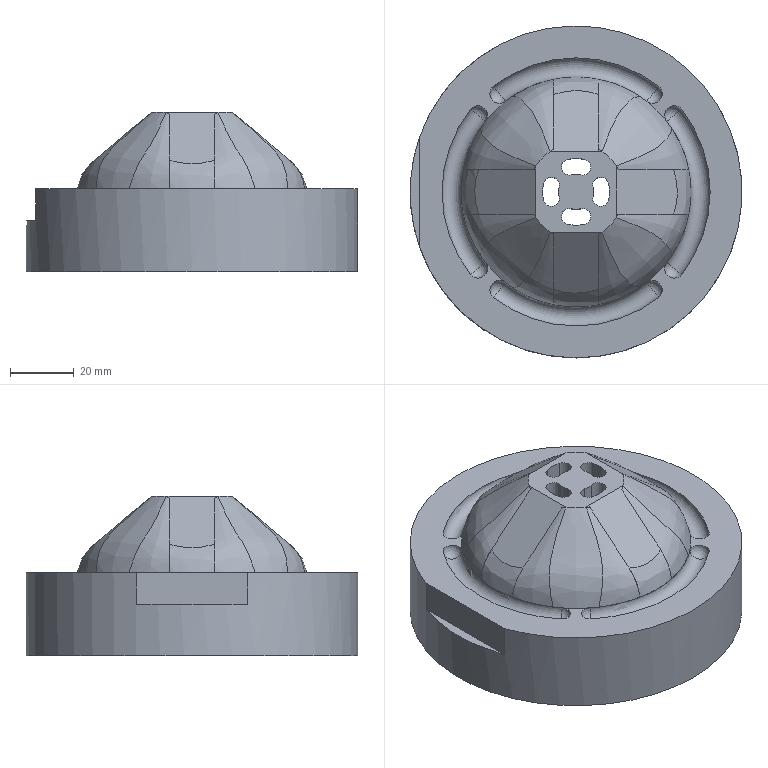NC program | NX | posted with a generic post | part box 104 x 104 x 49.86 mm
Lines 1 to 886 of 41131:
N10 G17 G21 G94 G90
(CAVITY_MILL , TOOL : D20R0.8)
N12 T00 M6
N14 G54
N16 G17 G0 G90 X-25.307 Y60.87 S2992 M3
N18 G43 Z20. H0
N20 Z-0.394
N22 G94 G1 Z-0.594 F1250.
N24 X-20.333 Y48.906
N26 G2 X26.248 Y46.008 R52.973 F2500.
N28 X51.613 Y-11.894 R52.996
N30 G1 X50.48 Y-16.058
N32 G2 X-38.754 Y-36.105 R52.977
N34 X-43.498 Y-30.233 R58.963
N36 X-20.333 Y48.906 R52.973
N38 G1 X-15.741 Y37.863
N40 G2 X20.32 Y35.62 R41.013
N42 X40.006 Y-8.998 R41.036
N44 G1 X39.011 Y-12.657
N46 G2 X-29.978 Y-27.979 R41.017
N48 X-33.704 Y-23.369 R47.003
N50 X-15.741 Y37.863 R41.013
N52 G1 X-11.15 Y26.819
N54 G2 X14.392 Y25.233 R29.053
N56 X28.389 Y-6.14 R29.076
N58 G1 X27.553 Y-9.214
N60 G2 X-21.203 Y-19.853 R29.057
N62 X-23.909 Y-16.505 R35.043
N64 X-11.15 Y26.819 R29.053
N66 G1 X-10.379 Y22.906
N68 G2 X-8.681 Y23.071 R8.786
N70 G1 X8.658
N72 G2 X13.35 Y21.729 R8.871
N74 X21.749 Y13.316 R26.19
N76 X23.071 Y8.681 R8.788
N78 G1 Y-8.663
N80 G2 X21.734 Y-13.342 R8.857
N82 X13.308 Y-21.754 R26.163
N84 X8.685 Y-23.071 R8.772
N86 G1 X-8.658
N88 G2 X-13.35 Y-21.729 R8.871
N90 X-21.749 Y-13.316 R26.19
N92 X-23.071 Y-8.681 R8.788
N94 G1 Y8.686
N96 G2 X-21.754 Y13.309 R8.769
N98 X-13.315 Y21.75 R26.175
N100 X-10.379 Y22.906 R8.786
N102 G3 X-4.863 Y31.126 R7.
N104 G1 X-11.113 Y71.102
N106 Z-0.394
N108 G0 Z0.3
N110 G1 X-25.307 Y60.87 F5000.
N112 G0 Z-0.988
N114 G1 Z-1.188 F1250.
N116 X-20.353 Y48.929
N118 G2 X9.52 Y52.133 R53.179 F2500.
N120 X29.214 Y44.212 R53.094
N122 X40.074 Y34.681 R53.73
N124 X52.332 Y-8.325 R53.011
N126 G1 X51.585 Y-12.117
N128 X50.507 Y-16.064
N130 G2 X-52.784 Y4.709 R52.998
N132 X-39.002 Y35.87 R52.95
N134 X-34.07 Y40.592 R54.178
N136 X-25.024 Y46.719 R56.698
N138 X-20.353 Y48.929 R53.179
N140 G1 X-15.77 Y37.882
N142 G2 X7.375 Y40.367 R41.219
N144 X22.614 Y34.238 R41.134
N146 X31.038 Y26.846 R41.77
N148 X40.553 Y-6.242 R41.051
N150 G1 X39.934 Y-9.381
N152 X39.039 Y-12.659
N154 G2 X-40.871 Y3.647 R41.038
N156 X-30.202 Y27.77 R40.99
N158 X-26.399 Y31.416 R42.218
N160 X-19.347 Y36.193 R44.738
N162 X-15.77 Y37.882 R41.219
N164 G1 X-11.188 Y26.835
N166 G2 X5.23 Y28.601 R29.259
N168 X16.014 Y24.264 R29.174
N170 X22.002 Y19.011 R29.81
N172 X28.766 Y-4.196 R29.091
N174 G1 X28.283 Y-6.645
N176 X27.582 Y-9.212
N178 G2 X-28.959 Y2.586 R29.078
N180 X-21.402 Y19.67 R29.03
N182 X-18.728 Y22.24 R30.258
N184 X-13.67 Y25.666 R32.778
N186 X-11.188 Y26.835 R29.259
N188 G1 X-10.509 Y23.631
N190 G2 X-6.468 Y23.779 R11.801
N192 G1 X6.453
N194 G2 X13.099 Y22.76 R11.911
N196 X22.76 Y13.099 R26.82
N198 X23.779 Y6.468 R11.801
N200 G1 Y-6.453
N202 G2 X22.76 Y-13.099 R11.911
N204 X13.099 Y-22.76 R26.82
N206 X6.468 Y-23.779 R11.801
N208 G1 X-6.453
N210 G2 X-13.099 Y-22.76 R11.911
N212 X-22.76 Y-13.099 R26.82
N214 X-23.779 Y-6.468 R11.801
N216 G1 Y6.453
N218 G2 X-22.76 Y13.099 R11.911
N220 X-13.099 Y22.76 R26.82
N222 X-10.509 Y23.631 R11.801
N224 G3 X-5.111 Y31.93 R7.
N226 G1 X-11.371 Y71.083
N228 Z-0.988
N230 G0 Z-0.294
N232 G1 X-25.307 Y60.87 F5000.
N234 G0 Z-1.582
N236 G1 Z-1.782 F1250.
N238 X-20.353 Y48.929
N240 G2 X9.52 Y52.133 R53.179 F2500.
N242 X29.214 Y44.212 R53.094
N244 X40.074 Y34.681 R53.73
N246 X52.332 Y-8.325 R53.011
N248 G1 X51.585 Y-12.117
N250 X50.507 Y-16.064
N252 G2 X-52.784 Y4.709 R52.998
N254 X-39.002 Y35.87 R52.95
N256 X-34.07 Y40.592 R54.178
N258 X-25.024 Y46.719 R56.698
N260 X-20.353 Y48.929 R53.179
N262 G1 X-15.77 Y37.882
N264 G2 X7.375 Y40.367 R41.219
N266 X22.614 Y34.238 R41.134
N268 X31.038 Y26.846 R41.77
N270 X40.553 Y-6.242 R41.051
N272 G1 X39.934 Y-9.381
N274 X39.039 Y-12.659
N276 G2 X37.457 Y-16.768 R41.038
N278 G1 X26.542 Y-11.88
N280 G3 X26.879 Y-6.148 R14.969
N282 G1 Y6.149
N284 G3 X26.553 Y11.841 R14.936
N286 G2 X28.766 Y-4.196 R29.091
N288 G1 X28.283 Y-6.645
N290 X27.582 Y-9.212
N292 G2 X26.542 Y-11.88 R29.077
N294 G1 X37.457 Y-16.768
N296 G2 X-16.701 Y-37.478 R41.038
N298 G1 X-11.833 Y-26.554
N300 G3 X-6.148 Y-26.879 R14.969
N302 G1 X6.149
N304 G3 X11.847 Y-26.551 R14.936
N306 G1 X21.681 Y-21.708
N308 X11.847 Y-26.551
N310 G2 X-11.833 Y-26.554 R29.078
N312 G1 X-21.693 Y-21.688
N314 X-11.833 Y-26.554
N316 X-16.701 Y-37.478
N318 G2 X-40.871 Y3.647 R41.038
N320 X-37.471 Y16.722 R40.99
N322 G1 X-26.55 Y11.846
N324 G3 X-26.879 Y6.148 R14.969
N326 G1 Y-6.149
N328 G3 X-26.555 Y-11.831 R14.936
N330 G2 X-28.959 Y2.586 R29.078
N332 X-26.55 Y11.846 R29.03
N334 G1 X-21.69 Y21.692
N336 X-26.55 Y11.846
N338 X-37.471 Y16.722
N340 G2 X-30.202 Y27.77 R40.99
N342 X-26.399 Y31.416 R42.218
N344 X-19.347 Y36.193 R44.738
N346 X-15.77 Y37.882 R41.219
N348 G1 X-11.188 Y26.835
N350 G2 X5.23 Y28.601 R29.259
N352 X11.825 Y26.558 R29.174
N354 G1 X21.687 Y21.695
N356 X11.825 Y26.558
N358 G3 X6.146 Y26.879 R14.907
N360 G1 X-6.149
N362 G3 X-11.848 Y26.551 R14.936
N364 G1 X-11.257 Y24.233
N366 G2 X-6.317 Y24.487 R12.544
N368 G1 X6.316
N370 G2 X13.099 Y23.608 R12.515
N372 X19.538 Y18.556 R25.887
N374 X23.608 Y13.099 R25.007
N376 X24.487 Y6.317 R12.544
N378 G1 Y-6.316
N380 G2 X23.608 Y-13.099 R12.577
N382 X18.556 Y-19.538 R25.887
N384 X13.099 Y-23.608 R25.007
N386 X6.317 Y-24.487 R12.544
N388 G1 X-6.316
N390 G2 X-13.099 Y-23.608 R12.577
N392 X-19.538 Y-18.556 R25.887
N394 X-23.608 Y-13.099 R25.007
N396 X-24.487 Y-6.317 R12.544
N398 G1 Y6.316
N400 G2 X-23.608 Y13.099 R12.577
N402 X-18.556 Y19.538 R25.887
N404 X-13.099 Y23.608 R25.007
N406 X-11.257 Y24.233 R12.544
N408 G1 X-11.848 Y26.551
N410 G2 X-11.188 Y26.835 R29.259
N412 G3 X-7.404 Y35.983 R7.
N414 G1 X-14.495 Y70.513
N416 Z-1.582
N418 G0 Z-0.888
N420 G1 X-25.307 Y60.87 F5000.
N422 G0 Z-2.176
N424 G1 Z-2.376 F1250.
N426 X-20.353 Y48.929
N428 G2 X9.52 Y52.133 R53.179 F2500.
N430 X29.214 Y44.212 R53.094
N432 X40.074 Y34.681 R53.73
N434 X52.332 Y-8.325 R53.011
N436 G1 X51.585 Y-12.117
N438 X50.507 Y-16.064
N440 G2 X-52.784 Y4.709 R52.998
N442 X-39.002 Y35.87 R52.95
N444 X-34.07 Y40.592 R54.178
N446 X-25.024 Y46.719 R56.698
N448 X-20.353 Y48.929 R53.179
N450 G1 X-15.77 Y37.882
N452 G2 X7.375 Y40.367 R41.219
N454 X12.246 Y39.163 R41.134
N456 G1 X8.672 Y27.749
N458 G3 X6.039 Y27.587 R14.932
N460 G1 X-6.07
N462 G3 X-8.791 Y27.708 R18.71
N464 G2 X5.23 Y28.601 R29.259
N466 X8.672 Y27.749 R29.174
N468 G1 X21.735 Y21.834
N470 X8.672 Y27.749
N472 X12.246 Y39.163
N474 G2 X22.614 Y34.238 R41.134
N476 X31.038 Y26.846 R41.77
N478 X40.553 Y-6.242 R41.051
N480 G1 X39.934 Y-9.381
N482 X39.288 Y-11.745
N484 X27.751 Y-8.594
N486 G3 X27.587 Y-6.039 R14.932
N488 G1 Y6.07
N490 G3 X27.708 Y8.801 R18.71
N492 G2 X28.766 Y-4.196 R29.091
N494 G1 X28.283 Y-6.645
N496 X27.751 Y-8.594
N498 X39.288 Y-11.745
N500 X39.039 Y-12.659
N502 G2 X-12.233 Y-39.165 R41.038
N504 G1 X-8.667 Y-27.749
N506 G3 X-6.039 Y-27.587 R14.932
N508 G1 X6.07
N510 G3 X8.806 Y-27.708 R18.71
N512 G1 X21.871 Y-21.699
N514 X8.806 Y-27.708
N516 G2 X-8.667 Y-27.749 R29.078
N518 G1 X-21.729 Y-21.84
N520 X-8.667 Y-27.749
N522 X-12.233 Y-39.165
N524 G2 X-40.871 Y3.647 R41.038
N526 X-39.163 Y12.248 R40.99
N528 G1 X-27.749 Y8.677
N530 G3 X-27.587 Y6.039 R14.932
N532 G1 Y-6.07
N534 G3 X-27.708 Y-8.8 R18.71
N536 G1 X-25.317 Y-8.731
N538 G2 X-25.195 Y-6.216 R16.318
N540 G1 Y6.226
N542 G2 X-24.014 Y13.927 R12.54
N544 X-14.394 Y23.741 R31.514
N546 X-10.725 Y25.137 R9.325
N548 X-6.216 Y25.195 R16.318
N550 G1 X6.226
N552 G2 X13.927 Y24.014 R12.54
N554 X23.741 Y14.394 R31.514
N556 X25.137 Y10.725 R9.325
N558 X25.195 Y6.216 R16.318
N560 G1 Y-6.226
N562 G2 X24.014 Y-13.927 R12.54
N564 X14.394 Y-23.741 R31.514
N566 X10.725 Y-25.137 R9.325
N568 X6.216 Y-25.195 R16.318
N570 G1 X-6.226
N572 G2 X-13.927 Y-24.014 R12.54
N574 X-23.741 Y-14.394 R31.514
N576 X-25.137 Y-10.725 R9.325
N578 X-25.317 Y-8.731 R16.318
N580 G1 X-27.708 Y-8.8
N582 G2 X-28.959 Y2.586 R29.078
N584 X-27.749 Y8.677 R29.03
N586 G1 X-21.836 Y21.731
N588 X-27.749 Y8.677
N590 X-39.163 Y12.248
N592 G2 X-30.202 Y27.77 R40.99
N594 X-26.399 Y31.416 R42.218
N596 X-19.347 Y36.193 R44.738
N598 X-15.77 Y37.882 R41.219
N600 G3 X-11.987 Y47.03 R7.
N602 G1 X-21.038 Y68.847
N604 Z-2.176
N606 G0 Z-1.482
N608 G1 X-25.307 Y60.87 F5000.
N610 G0 Z-2.77
N612 G1 Z-2.97 F1250.
N614 X-20.353 Y48.929
N616 G2 X9.52 Y52.133 R53.179 F2500.
N618 X29.214 Y44.212 R53.094
N620 X40.074 Y34.681 R53.73
N622 X52.332 Y-8.325 R53.011
N624 G1 X51.585 Y-12.117
N626 X50.507 Y-16.064
N628 G2 X-52.784 Y4.709 R52.998
N630 X-39.002 Y35.87 R52.95
N632 X-34.07 Y40.592 R54.178
N634 X-25.024 Y46.719 R56.698
N636 X-20.353 Y48.929 R53.179
N638 G1 X-15.77 Y37.882
N640 G2 X7.375 Y40.367 R41.219
N642 X9.127 Y40.006 R41.134
N644 G1 X6.46 Y28.348
N646 G3 X6.034 Y28.295 R16.746
N648 G1 X-6.028
N650 G3 X-6.452 Y28.342 R18.538
N652 G2 X5.23 Y28.601 R29.259
N654 X6.46 Y28.348 R29.174
N656 G1 X21.906 Y21.889
N658 X6.46 Y28.348
N660 X9.127 Y40.006
N662 G2 X22.614 Y34.238 R41.134
N664 X31.038 Y26.846 R41.77
N666 X40.553 Y-6.242 R41.051
N668 G1 X40.072 Y-8.683
N670 X28.337 Y-6.37
N672 G3 X28.295 Y-6.034 R16.746
N674 G1 Y6.028
N676 G3 X28.344 Y6.465 R18.538
N678 G2 X28.766 Y-4.196 R29.091
N680 G1 X28.337 Y-6.37
N682 X40.072 Y-8.683
N684 X39.934 Y-9.381
N686 X39.039 Y-12.659
N688 G2 X-9.106 Y-40.008 R41.038
N690 G1 X-6.451 Y-28.347
N692 G3 X-6.034 Y-28.295 R16.746
N694 G1 X6.028
N696 G3 X6.47 Y-28.344 R18.538
N698 G1 X21.931 Y-21.863
N700 X6.47 Y-28.344
N702 G2 X-6.451 Y-28.347 R29.077
N704 G1 X-21.895 Y-21.899
N706 X-6.451 Y-28.347
N708 X-9.106 Y-40.008
N710 G2 X-40.871 Y3.647 R41.038
N712 X-40.009 Y9.117 R40.99
N714 G1 X-28.348 Y6.46
N716 G3 X-28.295 Y6.034 R16.746
N718 G1 Y-6.028
N720 G3 X-28.344 Y-6.467 R18.538
N722 G1 X-25.964 Y-6.704
N724 G2 X-25.903 Y-6.181 R16.146
N726 G1 Y6.203
N728 G2 X-25.234 Y13.099 R14.354
N730 X-24.247 Y14.969 R7.318
N732 G1 X-23.532 Y15.949
N734 G2 X-15.106 Y24.14 R34.922
N736 X-10.846 Y25.842 R10.411
N738 X-6.181 Y25.903 R16.146
N740 G1 X6.203
N742 G2 X13.099 Y25.234 R14.354
N744 X14.969 Y24.247 R7.318
N746 G1 X15.949 Y23.532
N748 G2 X24.14 Y15.106 R34.922
N750 X25.842 Y10.846 R10.411
N752 X25.903 Y6.181 R16.146
N754 G1 Y-6.203
N756 G2 X25.234 Y-13.099 R14.354
N758 X24.247 Y-14.969 R7.318
N760 G1 X23.532 Y-15.949
N762 G2 X15.106 Y-24.14 R34.922
N764 X10.846 Y-25.842 R10.411
N766 X6.181 Y-25.903 R16.146
N768 G1 X-6.203
N770 G2 X-13.099 Y-25.234 R14.354
N772 X-14.969 Y-24.247 R7.318
N774 G1 X-15.949 Y-23.532
N776 G2 X-24.14 Y-15.106 R34.922
N778 X-25.842 Y-10.846 R10.411
N780 X-25.964 Y-6.704 R16.146
N782 G1 X-28.344 Y-6.467
N784 G2 X-28.959 Y2.586 R29.078
N786 X-28.348 Y6.46 R29.03
N788 G1 X-21.901 Y21.891
N790 X-28.348 Y6.46
N792 X-40.009 Y9.117
N794 G2 X-30.202 Y27.77 R40.99
N796 X-26.399 Y31.416 R42.218
N798 X-19.347 Y36.193 R44.738
N800 X-15.77 Y37.882 R41.219
N802 G3 X-11.987 Y47.03 R7.
N804 G1 X-21.038 Y68.847
N806 Z-2.77
N808 G0 Z-2.076
N810 G1 X-25.307 Y60.87 F5000.
N812 G0 Z-3.364
N814 G1 Z-3.564 F1250.
N816 X-20.353 Y48.929
N818 G2 X9.52 Y52.133 R53.179 F2500.
N820 X29.214 Y44.212 R53.094
N822 X40.074 Y34.681 R53.73
N824 X52.332 Y-8.325 R53.011
N826 G1 X51.585 Y-12.117
N828 X50.507 Y-16.064
N830 G2 X-52.784 Y4.709 R52.998
N832 X-39.002 Y35.87 R52.95
N834 X-34.07 Y40.592 R54.178
N836 X-25.024 Y46.719 R56.698
N838 X-20.353 Y48.929 R53.179
N840 G1 X-15.77 Y37.882
N842 G2 X2.776 Y40.936 R41.219
N844 G1 X1.978 Y29.003
N846 X-1.929
N848 G2 X1.978 Y29.003 R29.259
N850 G1 X11.177 Y28.938
N852 G2 X15.18 Y27.705 R16.41
N854 X15.436 Y27.569 R2.392
N856 X27.569 Y15.436 R36.475
N858 X27.706 Y15.178 R2.392
N860 X28.934 Y11.188 R16.475
N862 X29.815 Y11.152 R9.2
N864 G3 X24.087 Y20.819 R31.851
N866 X17.537 Y26.566 R32.57
N868 X11.141 Y29.818 R31.934
N870 G2 X11.177 Y28.938 R9.2
N872 G1 X1.978 Y29.003
N874 X2.776 Y40.936
N876 G2 X7.375 Y40.367 R41.219
N878 X22.614 Y34.238 R41.134
N880 X31.038 Y26.846 R41.77
N882 X40.935 Y-2.799 R41.051
N884 G1 X29.003 Y-1.983
N886 Y1.988
N888 G2 X29.003 Y-1.983 R29.091
N890 G1 X28.937 Y-11.182
N892 G2 X27.705 Y-15.18 R16.41
N894 X27.569 Y-15.436 R2.392
N896 X15.436 Y-27.569 R36.475
N898 X15.178 Y-27.706 R2.392
N900 X11.213 Y-28.93 R16.475
N902 X11.178 Y-29.807 R9.2
N904 G3 X29.825 Y-11.146 R31.838
N906 G2 X28.937 Y-11.182 R9.2
N908 G1 X29.003 Y-1.983
N910 X40.935 Y-2.799
N912 G2 X40.553 Y-6.242 R41.051
N914 G1 X39.934 Y-9.381
N916 X39.039 Y-12.659
N918 G2 X-2.831 Y-40.934 R41.038
N920 G1 X-2.005 Y-29.003
N922 X2.013
N924 G2 X-2.005 Y-29.003 R29.077
N926 G1 X-2.831 Y-40.934
N928 G2 X-40.934 Y2.864 R41.038
N930 G1 X-29.003 Y2.031
N932 Y-2.02
N934 X-29.802 Y-11.185
N936 G3 X-11.17 Y-29.807 R31.838
N938 G2 X-11.205 Y-28.933 R9.2
N940 X-15.18 Y-27.705 R16.41
N942 X-15.436 Y-27.569 R2.392
N944 X-27.569 Y-15.436 R36.475
N946 X-27.706 Y-15.178 R2.392
N948 X-28.929 Y-11.22 R16.475
N950 X-29.802 Y-11.185 R9.2
N952 G1 X-29.003 Y-2.02
N954 X-26.611
N956 Y6.186
N958 G2 X-25.527 Y14.19 R14.018
N960 X-14.19 Y25.528 R34.083
N962 X-6.169 Y26.611 R14.083
N964 G1 X6.186
N966 G2 X14.19 Y25.527 R14.018
N968 X25.528 Y14.19 R34.083
N970 X26.611 Y6.169 R14.083
N972 G1 Y-6.186
N974 G2 X25.527 Y-14.19 R14.018
N976 X14.19 Y-25.528 R34.083
N978 X6.169 Y-26.611 R14.083
N980 G1 X-6.186
N982 G2 X-14.19 Y-25.527 R14.018
N984 X-25.528 Y-14.19 R34.083
N986 X-26.611 Y-6.169 R14.083
N988 G1 Y-2.02
N990 X-29.003
N992 G2 X-29.003 Y2.031 R29.077
N994 G1 X-28.929 Y11.23
N996 G2 X-27.705 Y15.18 R16.41
N998 X-27.569 Y15.436 R2.392
N1000 X-15.436 Y27.569 R36.475
N1002 X-15.178 Y27.706 R2.392
N1004 X-11.129 Y28.945 R16.475
N1006 X-11.091 Y29.837 R9.2
N1008 G3 X-14.98 Y28.095 R32.019
N1010 X-20.498 Y24.358 R35.538
N1012 X-23.433 Y21.539 R33.018
N1014 X-29.8 Y11.196 R31.79
N1016 G2 X-28.929 Y11.23 R9.2
N1018 G1 X-29.003 Y2.031
N1020 X-40.934 Y2.864
N1022 G2 X-40.871 Y3.647 R41.038
N1024 X-30.202 Y27.77 R40.99
N1026 X-26.399 Y31.416 R42.218
N1028 X-19.347 Y36.193 R44.738
N1030 X-15.77 Y37.882 R41.219
N1032 G3 X-11.987 Y47.03 R7.
N1034 G1 X-21.038 Y68.847
N1036 Z-3.364
N1038 G0 Z-2.67
N1040 G1 X-25.307 Y60.87 F5000.
N1042 G0 Z-3.958
N1044 G1 Z-4.158 F1250.
N1046 X-20.353 Y48.929
N1048 G2 X9.52 Y52.133 R53.179 F2500.
N1050 X29.214 Y44.212 R53.094
N1052 X40.074 Y34.681 R53.73
N1054 X52.332 Y-8.325 R53.011
N1056 G1 X51.585 Y-12.117
N1058 X50.507 Y-16.064
N1060 G2 X-52.784 Y4.709 R52.998
N1062 X-39.002 Y35.87 R52.95
N1064 X-34.07 Y40.592 R54.178
N1066 X-25.024 Y46.719 R56.698
N1068 X-20.353 Y48.929 R53.179
N1070 G1 X-15.77 Y37.882
N1072 G2 X7.375 Y40.367 R41.219
N1074 X22.614 Y34.238 R41.134
N1076 X31.038 Y26.846 R41.77
N1078 X40.553 Y-6.242 R41.051
N1080 G1 X39.934 Y-9.381
N1082 X39.039 Y-12.659
N1084 G2 X37.429 Y-16.831 R41.038
N1086 G1 X29.221 Y-13.138
N1088 G3 X29.711 Y-5.993 R16.886
N1090 G1 Y5.994
N1092 G3 X29.233 Y13.099 R16.887
N1094 G2 X31.684 Y-4.698 R32.051
N1096 G1 X31.167 Y-7.322
N1098 X30.416 Y-10.07
N1100 G2 X29.221 Y-13.138 R32.037
N1102 G1 X37.429 Y-16.831
N1104 G2 X-16.759 Y-37.452 R41.038
N1106 G1 X-13.083 Y-29.237
N1108 G3 X-5.993 Y-29.711 R16.886
N1110 G1 X5.994
N1112 G3 X13.105 Y-29.231 R16.887
N1114 G2 X-13.083 Y-29.237 R32.038
N1116 G1 X-16.759 Y-37.452
N1118 G2 X-40.871 Y3.647 R41.038
N1120 X-37.445 Y16.781 R40.99
N1122 G1 X-29.233 Y13.098
N1124 G3 X-29.711 Y5.993 R16.886
N1126 G1 Y-5.994
N1128 G3 X-29.237 Y-13.086 R16.887
N1130 G2 X-31.907 Y2.849 R32.037
N1132 X-29.233 Y13.098 R31.99
N1134 G1 X-37.445 Y16.781
N1136 G2 X-30.202 Y27.77 R40.99
N1138 X-26.399 Y31.416 R42.218
N1140 X-19.347 Y36.193 R44.738
N1142 X-15.77 Y37.882 R41.219
N1144 G1 X-12.322 Y29.569
N1146 G2 X5.76 Y31.513 R32.219
N1148 X13.086 Y29.236 R32.134
N1150 G3 X5.993 Y29.711 R16.886
N1152 G1 X-5.994
N1154 G3 X-13.108 Y29.23 R16.887
N1156 G1 X-12.446 Y26.932
N1158 G2 X-6.175 Y27.319 R14.495
N1160 G1 X6.174
N1162 G2 X14.437 Y26.197 R14.494
N1164 X21.264 Y20.739 R32.312
N1166 X26.197 Y14.437 R31.95
N1168 X27.319 Y6.175 R14.495
N1170 G1 Y-6.174
N1172 G2 X26.197 Y-14.437 R14.494
N1174 X20.739 Y-21.264 R32.312
N1176 X14.437 Y-26.197 R31.95
N1178 X6.175 Y-27.319 R14.495
N1180 G1 X-6.174
N1182 G2 X-14.437 Y-26.197 R14.494
N1184 X-21.264 Y-20.739 R32.312
N1186 X-26.197 Y-14.437 R31.95
N1188 X-27.319 Y-6.175 R14.495
N1190 G1 Y6.174
N1192 G2 X-26.197 Y14.437 R14.494
N1194 X-20.739 Y21.264 R32.312
N1196 X-14.437 Y26.197 R31.95
N1198 X-12.446 Y26.932 R14.495
N1200 G1 X-13.108 Y29.23
N1202 G2 X-12.322 Y29.569 R32.219
N1204 G3 X-8.538 Y38.717 R7.
N1206 G1 X-15.489 Y70.301
N1208 Z-3.958
N1210 G0 Z-3.264
N1212 G1 X-25.307 Y60.87 F5000.
N1214 G0 Z-4.552
N1216 G1 Z-4.752 F1250.
N1218 X-20.353 Y48.929
N1220 G2 X9.52 Y52.133 R53.179 F2500.
N1222 X29.214 Y44.212 R53.094
N1224 X40.074 Y34.681 R53.73
N1226 X52.332 Y-8.325 R53.011
N1228 G1 X51.585 Y-12.117
N1230 X50.507 Y-16.064
N1232 G2 X-52.784 Y4.709 R52.998
N1234 X-39.002 Y35.87 R52.95
N1236 X-34.07 Y40.592 R54.178
N1238 X-25.024 Y46.719 R56.698
N1240 X-20.353 Y48.929 R53.179
N1242 G1 X-15.77 Y37.882
N1244 G2 X7.375 Y40.367 R41.219
N1246 X12.345 Y39.132 R41.134
N1248 G1 X9.634 Y30.55
N1250 G3 X5.993 Y30.419 R18.009
N1252 G1 X-6.024
N1254 G3 X-9.635 Y30.546 R19.375
N1256 G2 X5.76 Y31.513 R32.219
N1258 X9.634 Y30.55 R32.134
N1260 G1 X12.345 Y39.132
N1262 G2 X22.614 Y34.238 R41.134
N1264 X31.038 Y26.846 R41.77
N1266 X40.553 Y-6.242 R41.051
N1268 G1 X39.934 Y-9.381
N1270 X39.236 Y-11.937
N1272 X30.554 Y-9.566
N1274 G3 X30.419 Y-5.993 R18.009
N1276 G1 Y6.024
N1278 G3 X30.545 Y9.646 R19.375
N1280 G2 X31.684 Y-4.698 R32.051
N1282 G1 X31.167 Y-7.322
N1284 X30.554 Y-9.566
N1286 X39.236 Y-11.937
N1288 X39.039 Y-12.659
N1290 G2 X-12.334 Y-39.134 R41.038
N1292 G1 X-9.628 Y-30.55
N1294 G3 X-5.993 Y-30.419 R18.009
N1296 G1 X6.024
N1298 G3 X9.652 Y-30.545 R19.375
N1300 G2 X-9.628 Y-30.55 R32.037
N1302 G1 X-12.334 Y-39.134
N1304 G2 X-40.871 Y3.647 R41.038
N1306 X-39.132 Y12.349 R40.99
N1308 G1 X-30.549 Y9.64
N1310 G3 X-30.419 Y5.993 R18.009
N1312 G1 Y-6.024
N1314 G3 X-30.546 Y-9.644 R19.375
N1316 G1 X-28.158 Y-9.505
N1318 G2 X-28.027 Y-6.184 R16.983
N1320 G1 Y6.164
N1322 G2 X-27.106 Y14.19 R15.617
N1324 X-25.592 Y16.684 R14.657
N1326 G1 X-25.004 Y17.465
N1328 G2 X-16.054 Y26.019 R39.967
N1330 X-11.234 Y27.967 R11.749
N1332 X-6.184 Y28.027 R16.983
N1334 G1 X6.164
N1336 G2 X14.19 Y27.106 R15.617
N1338 X16.684 Y25.592 R14.657
N1340 G1 X17.465 Y25.004
N1342 G2 X26.019 Y16.054 R39.967
N1344 X27.967 Y11.234 R11.749
N1346 X28.027 Y6.184 R16.983
N1348 G1 Y-6.164
N1350 G2 X27.106 Y-14.19 R15.617
N1352 X25.592 Y-16.684 R14.657
N1354 G1 X25.004 Y-17.465
N1356 G2 X16.054 Y-26.019 R39.967
N1358 X11.234 Y-27.967 R11.749
N1360 X6.184 Y-28.027 R16.983
N1362 G1 X-6.164
N1364 G2 X-14.19 Y-27.106 R15.617
N1366 X-16.684 Y-25.592 R14.657
N1368 G1 X-17.465 Y-25.004
N1370 G2 X-26.019 Y-16.054 R39.967
N1372 X-27.967 Y-11.234 R11.749
N1374 X-28.158 Y-9.505 R16.983
N1376 G1 X-30.546 Y-9.644
N1378 G2 X-31.907 Y2.849 R32.037
N1380 X-30.549 Y9.64 R31.99
N1382 G1 X-39.132 Y12.349
N1384 G2 X-30.202 Y27.77 R40.99
N1386 X-26.399 Y31.416 R42.218
N1388 X-19.347 Y36.193 R44.738
N1390 X-15.77 Y37.882 R41.219
N1392 G3 X-11.987 Y47.03 R7.
N1394 G1 X-21.038 Y68.847
N1396 Z-4.552
N1398 G0 Z-3.858
N1400 G1 X-25.307 Y60.87 F5000.
N1402 G0 Z-5.146
N1404 G1 Z-5.346 F1250.
N1406 X-20.353 Y48.929
N1408 G2 X9.52 Y52.133 R53.179 F2500.
N1410 X29.214 Y44.212 R53.094
N1412 X40.074 Y34.681 R53.73
N1414 X52.332 Y-8.325 R53.011
N1416 G1 X51.585 Y-12.117
N1418 X50.507 Y-16.064
N1420 G2 X-52.784 Y4.709 R52.998
N1422 X-39.002 Y35.87 R52.95
N1424 X-34.07 Y40.592 R54.178
N1426 X-25.024 Y46.719 R56.698
N1428 X-20.353 Y48.929 R53.179
N1430 G1 X-15.77 Y37.882
N1432 G2 X7.375 Y40.367 R41.219
N1434 X9.05 Y40.024 R41.134
N1436 G1 X7.06 Y31.247
N1438 G3 X5.98 Y31.126 R17.896
N1440 G1 X-6.029
N1442 G3 X-7.048 Y31.242 R17.737
N1444 G2 X5.76 Y31.513 R32.219
N1446 X7.06 Y31.247 R32.134
N1448 G1 X9.05 Y40.024
N1450 G2 X22.614 Y34.238 R41.134
N1452 X31.038 Y26.846 R41.77
N1454 X40.553 Y-6.242 R41.051
N1456 G1 X40.068 Y-8.699
N1458 X31.238 Y-6.959
N1460 G3 X31.126 Y-5.98 R17.896
N1462 G1 Y6.029
N1464 G3 X31.243 Y7.062 R17.737
N1466 G2 X31.684 Y-4.698 R32.051
N1468 G1 X31.238 Y-6.959
N1470 X40.068 Y-8.699
N1472 X39.934 Y-9.381
N1474 X39.039 Y-12.659
N1476 G2 X-9.032 Y-40.025 R41.038
N1478 G1 X-7.05 Y-31.246
N1480 G3 X-5.98 Y-31.126 R17.896
N1482 G1 X6.029
N1484 G3 X7.068 Y-31.244 R17.737
N1486 G2 X-7.05 Y-31.246 R32.037
N1488 G1 X-9.032 Y-40.025
N1490 G2 X-40.871 Y3.647 R41.038
N1492 X-40.025 Y9.043 R40.99
N1494 G1 X-31.247 Y7.059
N1496 G3 X-31.126 Y5.98 R17.896
N1498 G1 Y-6.029
N1500 G3 X-31.244 Y-7.064 R17.737
N1502 G1 X-28.86 Y-7.263
N1504 G2 X-28.734 Y-6.205 R15.345
N1506 G1 Y6.156
N1508 G2 X-27.352 Y15.282 R15.504
N1510 X-15.282 Y27.352 R40.53
N1512 X-6.205 Y28.734 R15.345
N1514 G1 X6.156
N1516 G2 X15.282 Y27.352 R15.504
N1518 X27.352 Y15.282 R40.53
N1520 X28.734 Y6.205 R15.345
N1522 G1 Y-6.156
N1524 G2 X27.352 Y-15.282 R15.504
N1526 X15.282 Y-27.352 R40.53
N1528 X6.205 Y-28.734 R15.345
N1530 G1 X-6.156
N1532 G2 X-15.282 Y-27.352 R15.504
N1534 X-27.352 Y-15.282 R40.53
N1536 X-28.86 Y-7.263 R15.345
N1538 G1 X-31.244 Y-7.064
N1540 G2 X-31.907 Y2.849 R32.038
N1542 X-31.247 Y7.059 R31.99
N1544 G1 X-40.025 Y9.043
N1546 G2 X-30.202 Y27.77 R40.99
N1548 X-26.399 Y31.416 R42.218
N1550 X-19.347 Y36.193 R44.738
N1552 X-15.77 Y37.882 R41.219
N1554 G3 X-11.987 Y47.03 R7.
N1556 G1 X-21.038 Y68.847
N1558 Z-5.146
N1560 G0 Z-4.452
N1562 G1 X-25.307 Y60.87 F5000.
N1564 G0 Z-5.74
N1566 G1 Z-5.94 F1250.
N1568 X-20.353 Y48.929
N1570 G2 X9.52 Y52.133 R53.179 F2500.
N1572 X29.214 Y44.212 R53.094
N1574 X40.074 Y34.681 R53.73
N1576 X52.332 Y-8.325 R53.011
N1578 G1 X51.585 Y-12.117
N1580 X50.507 Y-16.064
N1582 G2 X-52.784 Y4.709 R52.998
N1584 X-39.002 Y35.87 R52.95
N1586 X-34.07 Y40.592 R54.178
N1588 X-25.024 Y46.719 R56.698
N1590 X-20.353 Y48.929 R53.179
N1592 G1 X-15.77 Y37.882
N1594 G2 X4.536 Y40.78 R41.219
N1596 G1 X3.551 Y31.834
N1598 X-3.503
N1600 G2 X3.551 Y31.834 R32.219
N1602 G1 X4.536 Y40.78
N1604 G2 X7.375 Y40.367 R41.219
N1606 X22.614 Y34.238 R41.134
N1608 X31.038 Y26.846 R41.77
N1610 X40.779 Y-4.532 R41.051
N1612 G1 X31.834 Y-3.538
N1614 Y3.544
N1616 G2 X31.834 Y-3.538 R32.051
N1618 G1 X40.779 Y-4.532
N1620 G2 X40.553 Y-6.242 R41.051
N1622 G1 X39.934 Y-9.381
N1624 X39.039 Y-12.659
N1626 G2 X-4.55 Y-40.779 R41.038
N1628 G1 X-3.551 Y-31.834
N1630 X3.559
N1632 G2 X-3.551 Y-31.834 R32.038
N1634 G1 X-4.55 Y-40.779
N1636 G2 X-40.871 Y3.647 R41.038
N1638 X-40.778 Y4.572 R40.99
N1640 G1 X-31.834 Y3.57
N1642 Y-3.56
N1644 X-29.442
N1646 Y6.168
N1648 G2 X-28.142 Y15.282 R16.3
N1650 X-22.923 Y21.918 R36.304
N1652 X-15.282 Y28.142 R37.065
N1654 X-6.239 Y29.442 R16.12
N1656 G1 X6.168
N1658 G2 X15.282 Y28.142 R16.3
N1660 X21.918 Y22.923 R36.304
N1662 X28.142 Y15.282 R37.065
N1664 X29.442 Y6.239 R16.12
N1666 G1 Y-6.168
N1668 G2 X28.142 Y-15.282 R16.3
N1670 X22.923 Y-21.918 R36.304
N1672 X15.282 Y-28.142 R37.065
N1674 X6.239 Y-29.442 R16.12
N1676 G1 X-6.168
N1678 G2 X-15.282 Y-28.142 R16.3
N1680 X-21.918 Y-22.923 R36.304
N1682 X-28.142 Y-15.282 R37.065
N1684 X-29.442 Y-6.239 R16.12
N1686 G1 Y-3.56
N1688 X-31.834
N1690 G2 X-31.907 Y2.849 R32.037
N1692 X-31.834 Y3.57 R31.99
N1694 G1 X-40.778 Y4.572
N1696 G2 X-30.202 Y27.77 R40.99
N1698 X-26.399 Y31.416 R42.218
N1700 X-19.347 Y36.193 R44.738
N1702 X-15.77 Y37.882 R41.219
N1704 G3 X-11.987 Y47.03 R7.
N1706 G1 X-21.038 Y68.847
N1708 Z-5.74
N1710 G0 Z-5.046
N1712 G1 X-25.307 Y60.87 F5000.
N1714 G0 Z-6.334
N1716 G1 Z-6.534 F1250.
N1718 X-20.353 Y48.929
N1720 G2 X9.52 Y52.133 R53.179 F2500.
N1722 X29.214 Y44.212 R53.094
N1724 X40.074 Y34.681 R53.73
N1726 X52.332 Y-8.325 R53.011
N1728 G1 X51.585 Y-12.117
N1730 X50.507 Y-16.064
N1732 G2 X-52.784 Y4.709 R52.998
N1734 X-39.002 Y35.87 R52.95
N1736 X-34.07 Y40.592 R54.178
N1738 X-25.024 Y46.719 R56.698
N1740 X-20.353 Y48.929 R53.179
N1742 G1 X-15.77 Y37.882
N1744 G2 X7.375 Y40.367 R41.219
N1746 X22.614 Y34.238 R41.134
N1748 X31.038 Y26.846 R41.77
N1750 X40.553 Y-6.242 R41.051
N1752 G1 X39.934 Y-9.381
N1754 X39.039 Y-12.659
N1756 G2 X-40.871 Y3.647 R41.038
N1758 X-30.202 Y27.77 R40.99
N1760 X-26.399 Y31.416 R42.218
N1762 X-19.347 Y36.193 R44.738
N1764 X-15.77 Y37.882 R41.219
N1766 G1 X-13.35 Y29.641
N1768 G2 X-12.007 Y29.959 R12.967
N1770 G1 X-11.369 Y30.068